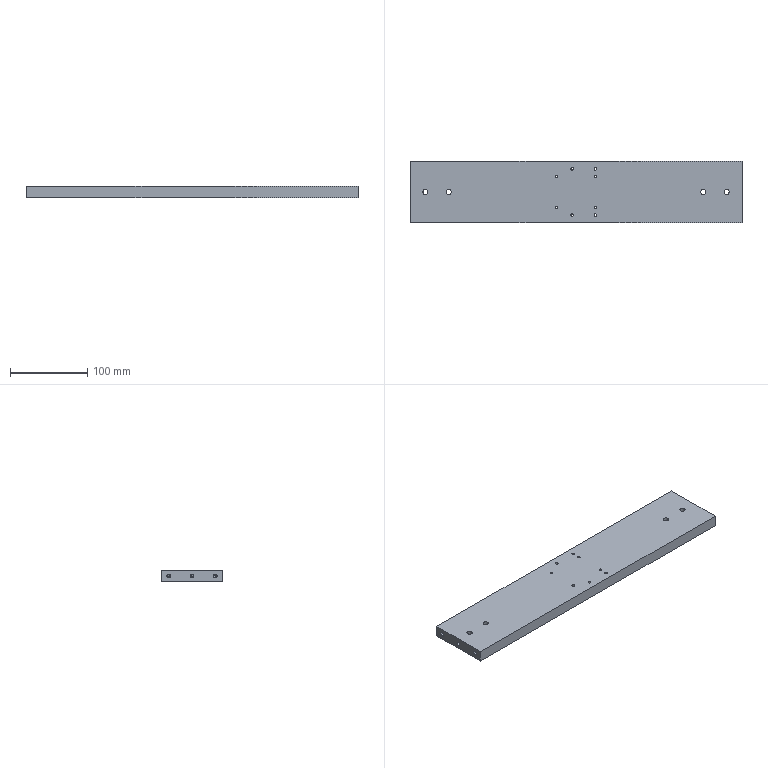Part | SolidWorks | features HoleWzd 5, Extrusion 1, MirrorPattern 1 | 1 solid | 62 faces | box 430 x 80 x 15 mm | volume 509108 mm3 | cylinder 44 | plane 10 | cone 8 | commonest cylinder face diameters 3.3 x16 5 x12 6.6 x8 11 x8